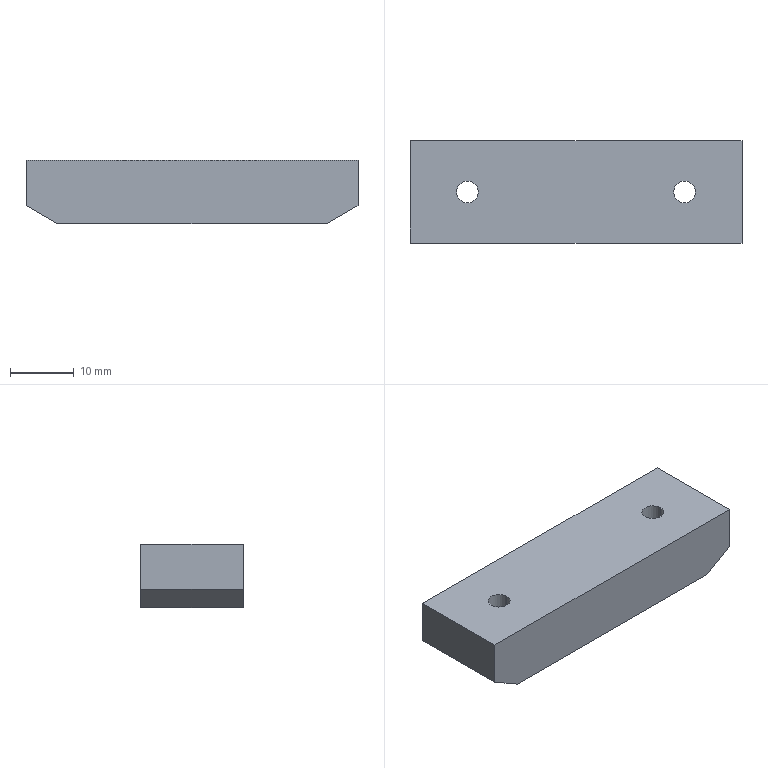Part | SolidWorks | features Chamfer 2, Extrusion 1, HoleWzd 1 | 1 solid | 18 faces | box 52 x 16 x 10 mm | volume 7777 mm3 | plane 10 | cylinder 8 | commonest cylinder face diameters 3.4 x4 6 x4
STEP:
#1=CARTESIAN_POINT('',(20.,0.,3.4));
#2=VERTEX_POINT('',#1);
#3=CARTESIAN_POINT('',(14.,0.,3.4));
#4=VERTEX_POINT('',#3);
#5=CARTESIAN_POINT('',(17.,0.,3.4));
#6=DIRECTION('',(0.,0.,-1.));
#7=DIRECTION('',(-1.,0.,0.));
#8=AXIS2_PLACEMENT_3D('',#5,#6,#7);
#9=CIRCLE('',#8,3.);
#10=EDGE_CURVE('',#2,#4,#9,.T.);
#11=ORIENTED_EDGE('',*,*,#10,.F.);
#12=CARTESIAN_POINT('',(20.,0.,0.));
#13=VERTEX_POINT('',#12);
#14=CARTESIAN_POINT('',(20.,0.,0.));
#15=DIRECTION('',(0.,0.,-1.));
#16=VECTOR('',#15,1000.);
#17=LINE('',#14,#16);
#18=EDGE_CURVE('',#2,#13,#17,.T.);
#19=ORIENTED_EDGE('',*,*,#18,.T.);
#20=CARTESIAN_POINT('',(14.,0.,0.));
#21=VERTEX_POINT('',#20);
#22=CARTESIAN_POINT('',(17.,0.,0.));
#23=DIRECTION('',(0.,0.,-1.));
#24=DIRECTION('',(-1.,0.,0.));
#25=AXIS2_PLACEMENT_3D('',#22,#23,#24);
#26=CIRCLE('',#25,3.);
#27=EDGE_CURVE('',#13,#21,#26,.T.);
#28=ORIENTED_EDGE('',*,*,#27,.T.);
#29=CARTESIAN_POINT('',(14.,0.,0.));
#30=DIRECTION('',(0.,0.,-1.));
#31=VECTOR('',#30,1000.);
#32=LINE('',#29,#31);
#33=EDGE_CURVE('',#4,#21,#32,.T.);
#34=ORIENTED_EDGE('',*,*,#33,.F.);
#35=EDGE_LOOP('',(#11,#19,#28,#34));
#36=FACE_OUTER_BOUND('',#35,.T.);
#37=CARTESIAN_POINT('',(17.,0.,0.));
#38=DIRECTION('',(0.,0.,-1.));
#39=DIRECTION('',(-1.,0.,0.));
#40=AXIS2_PLACEMENT_3D('',#37,#38,#39);
#41=CYLINDRICAL_SURFACE('',#40,3.);
#42=ADVANCED_FACE('',(#36),#41,.F.);
#43=CARTESIAN_POINT('',(15.3,0.,10.));
#44=VERTEX_POINT('',#43);
#45=CARTESIAN_POINT('',(18.7,0.,10.));
#46=VERTEX_POINT('',#45);
#47=CARTESIAN_POINT('',(17.,0.,10.));
#48=DIRECTION('',(0.,0.,1.));
#49=DIRECTION('',(1.,0.,0.));
#50=AXIS2_PLACEMENT_3D('',#47,#48,#49);
#51=CIRCLE('',#50,1.7);
#52=EDGE_CURVE('',#44,#46,#51,.T.);
#53=ORIENTED_EDGE('',*,*,#52,.T.);
#54=CARTESIAN_POINT('',(18.7,0.,3.4));
#55=VERTEX_POINT('',#54);
#56=CARTESIAN_POINT('',(18.7,0.,0.));
#57=DIRECTION('',(0.,0.,-1.));
#58=VECTOR('',#57,1000.);
#59=LINE('',#56,#58);
#60=EDGE_CURVE('',#46,#55,#59,.T.);
#61=ORIENTED_EDGE('',*,*,#60,.T.);
#62=CARTESIAN_POINT('',(15.3,0.,3.4));
#63=VERTEX_POINT('',#62);
#64=CARTESIAN_POINT('',(17.,0.,3.4));
#65=DIRECTION('',(0.,0.,-1.));
#66=DIRECTION('',(-1.,0.,0.));
#67=AXIS2_PLACEMENT_3D('',#64,#65,#66);
#68=CIRCLE('',#67,1.7);
#69=EDGE_CURVE('',#55,#63,#68,.T.);
#70=ORIENTED_EDGE('',*,*,#69,.T.);
#71=CARTESIAN_POINT('',(15.3,0.,0.));
#72=DIRECTION('',(0.,0.,-1.));
#73=VECTOR('',#72,1000.);
#74=LINE('',#71,#73);
#75=EDGE_CURVE('',#44,#63,#74,.T.);
#76=ORIENTED_EDGE('',*,*,#75,.F.);
#77=EDGE_LOOP('',(#53,#61,#70,#76));
#78=FACE_OUTER_BOUND('',#77,.T.);
#79=CARTESIAN_POINT('',(17.,0.,0.));
#80=DIRECTION('',(0.,0.,-1.));
#81=DIRECTION('',(-1.,0.,0.));
#82=AXIS2_PLACEMENT_3D('',#79,#80,#81);
#83=CYLINDRICAL_SURFACE('',#82,1.7);
#84=ADVANCED_FACE('',(#78),#83,.F.);
#85=CARTESIAN_POINT('',(-14.,0.,3.4));
#86=VERTEX_POINT('',#85);
#87=CARTESIAN_POINT('',(-20.,0.,3.4));
#88=VERTEX_POINT('',#87);
#89=CARTESIAN_POINT('',(-17.,0.,3.4));
#90=DIRECTION('',(0.,0.,-1.));
#91=DIRECTION('',(-1.,0.,0.));
#92=AXIS2_PLACEMENT_3D('',#89,#90,#91);
#93=CIRCLE('',#92,3.);
#94=EDGE_CURVE('',#86,#88,#93,.T.);
#95=ORIENTED_EDGE('',*,*,#94,.F.);
#96=CARTESIAN_POINT('',(-14.,0.,0.));
#97=VERTEX_POINT('',#96);
#98=CARTESIAN_POINT('',(-14.,0.,0.));
#99=DIRECTION('',(0.,0.,-1.));
#100=VECTOR('',#99,1000.);
#101=LINE('',#98,#100);
#102=EDGE_CURVE('',#86,#97,#101,.T.);
#103=ORIENTED_EDGE('',*,*,#102,.T.);
#104=CARTESIAN_POINT('',(-20.,0.,0.));
#105=VERTEX_POINT('',#104);
#106=CARTESIAN_POINT('',(-17.,0.,0.));
#107=DIRECTION('',(0.,0.,-1.));
#108=DIRECTION('',(-1.,0.,0.));
#109=AXIS2_PLACEMENT_3D('',#106,#107,#108);
#110=CIRCLE('',#109,3.);
#111=EDGE_CURVE('',#97,#105,#110,.T.);
#112=ORIENTED_EDGE('',*,*,#111,.T.);
#113=CARTESIAN_POINT('',(-20.,0.,0.));
#114=DIRECTION('',(0.,0.,-1.));
#115=VECTOR('',#114,1000.);
#116=LINE('',#113,#115);
#117=EDGE_CURVE('',#88,#105,#116,.T.);
#118=ORIENTED_EDGE('',*,*,#117,.F.);
#119=EDGE_LOOP('',(#95,#103,#112,#118));
#120=FACE_OUTER_BOUND('',#119,.T.);
#121=CARTESIAN_POINT('',(-17.,0.,0.));
#122=DIRECTION('',(0.,0.,-1.));
#123=DIRECTION('',(-1.,0.,0.));
#124=AXIS2_PLACEMENT_3D('',#121,#122,#123);
#125=CYLINDRICAL_SURFACE('',#124,3.);
#126=ADVANCED_FACE('',(#120),#125,.F.);
#127=CARTESIAN_POINT('',(-18.7,0.,10.));
#128=VERTEX_POINT('',#127);
#129=CARTESIAN_POINT('',(-15.3,0.,10.));
#130=VERTEX_POINT('',#129);
#131=CARTESIAN_POINT('',(-17.,0.,10.));
#132=DIRECTION('',(0.,0.,1.));
#133=DIRECTION('',(1.,0.,0.));
#134=AXIS2_PLACEMENT_3D('',#131,#132,#133);
#135=CIRCLE('',#134,1.7);
#136=EDGE_CURVE('',#128,#130,#135,.T.);
#137=ORIENTED_EDGE('',*,*,#136,.T.);
#138=CARTESIAN_POINT('',(-15.3,0.,3.4));
#139=VERTEX_POINT('',#138);
#140=CARTESIAN_POINT('',(-15.3,0.,0.));
#141=DIRECTION('',(0.,0.,-1.));
#142=VECTOR('',#141,1000.);
#143=LINE('',#140,#142);
#144=EDGE_CURVE('',#130,#139,#143,.T.);
#145=ORIENTED_EDGE('',*,*,#144,.T.);
#146=CARTESIAN_POINT('',(-18.7,0.,3.4));
#147=VERTEX_POINT('',#146);
#148=CARTESIAN_POINT('',(-17.,0.,3.4));
#149=DIRECTION('',(0.,0.,-1.));
#150=DIRECTION('',(-1.,0.,0.));
#151=AXIS2_PLACEMENT_3D('',#148,#149,#150);
#152=CIRCLE('',#151,1.7);
#153=EDGE_CURVE('',#139,#147,#152,.T.);
#154=ORIENTED_EDGE('',*,*,#153,.T.);
#155=CARTESIAN_POINT('',(-18.7,0.,0.));
#156=DIRECTION('',(0.,0.,-1.));
#157=VECTOR('',#156,1000.);
#158=LINE('',#155,#157);
#159=EDGE_CURVE('',#128,#147,#158,.T.);
#160=ORIENTED_EDGE('',*,*,#159,.F.);
#161=EDGE_LOOP('',(#137,#145,#154,#160));
#162=FACE_OUTER_BOUND('',#161,.T.);
#163=CARTESIAN_POINT('',(-17.,0.,0.));
#164=DIRECTION('',(0.,0.,-1.));
#165=DIRECTION('',(-1.,0.,0.));
#166=AXIS2_PLACEMENT_3D('',#163,#164,#165);
#167=CYLINDRICAL_SURFACE('',#166,1.7);
#168=ADVANCED_FACE('',(#162),#167,.F.);
#169=CARTESIAN_POINT('',(-26.,8.,10.));
#170=VERTEX_POINT('',#169);
#171=CARTESIAN_POINT('',(-26.,8.,2.887));
#172=VERTEX_POINT('',#171);
#173=CARTESIAN_POINT('',(-26.,8.,10.));
#174=DIRECTION('',(0.,0.,-1.));
#175=VECTOR('',#174,1000.);
#176=LINE('',#173,#175);
#177=EDGE_CURVE('',#170,#172,#176,.T.);
#178=ORIENTED_EDGE('',*,*,#177,.T.);
#179=CARTESIAN_POINT('',(-26.,-8.,2.887));
#180=VERTEX_POINT('',#179);
#181=CARTESIAN_POINT('',(-26.,-8.,2.887));
#182=DIRECTION('',(0.,-1.,0.));
#183=VECTOR('',#182,1000.);
#184=LINE('',#181,#183);
#185=EDGE_CURVE('',#172,#180,#184,.T.);
#186=ORIENTED_EDGE('',*,*,#185,.T.);
#187=CARTESIAN_POINT('',(-26.,-8.,10.));
#188=VERTEX_POINT('',#187);
#189=CARTESIAN_POINT('',(-26.,-8.,10.));
#190=DIRECTION('',(0.,0.,-1.));
#191=VECTOR('',#190,1000.);
#192=LINE('',#189,#191);
#193=EDGE_CURVE('',#188,#180,#192,.T.);
#194=ORIENTED_EDGE('',*,*,#193,.F.);
#195=CARTESIAN_POINT('',(-26.,-8.,10.));
#196=DIRECTION('',(0.,-1.,0.));
#197=VECTOR('',#196,1000.);
#198=LINE('',#195,#197);
#199=EDGE_CURVE('',#170,#188,#198,.T.);
#200=ORIENTED_EDGE('',*,*,#199,.F.);
#201=EDGE_LOOP('',(#178,#186,#194,#200));
#202=FACE_OUTER_BOUND('',#201,.T.);
#203=CARTESIAN_POINT('',(-26.,-8.,10.));
#204=DIRECTION('',(1.,0.,0.));
#205=DIRECTION('',(0.,0.,-1.));
#206=AXIS2_PLACEMENT_3D('',#203,#204,#205);
#207=PLANE('',#206);
#208=ADVANCED_FACE('',(#202),#207,.F.);
#209=ORIENTED_EDGE('',*,*,#193,.T.);
#210=CARTESIAN_POINT('',(-21.,-8.,0.));
#211=VERTEX_POINT('',#210);
#212=CARTESIAN_POINT('',(-26.,-8.,2.887));
#213=DIRECTION('',(0.866,0.,-0.5));
#214=VECTOR('',#213,1000.);
#215=LINE('',#212,#214);
#216=EDGE_CURVE('',#180,#211,#215,.T.);
#217=ORIENTED_EDGE('',*,*,#216,.T.);
#218=CARTESIAN_POINT('',(21.,-8.,0.));
#219=VERTEX_POINT('',#218);
#220=CARTESIAN_POINT('',(26.,-8.,0.));
#221=DIRECTION('',(1.,0.,0.));
#222=VECTOR('',#221,1000.);
#223=LINE('',#220,#222);
#224=EDGE_CURVE('',#211,#219,#223,.T.);
#225=ORIENTED_EDGE('',*,*,#224,.T.);
#226=CARTESIAN_POINT('',(26.,-8.,2.887));
#227=VERTEX_POINT('',#226);
#228=CARTESIAN_POINT('',(26.,-8.,2.887));
#229=DIRECTION('',(0.866,0.,0.5));
#230=VECTOR('',#229,1000.);
#231=LINE('',#228,#230);
#232=EDGE_CURVE('',#219,#227,#231,.T.);
#233=ORIENTED_EDGE('',*,*,#232,.T.);
#234=CARTESIAN_POINT('',(26.,-8.,10.));
#235=VERTEX_POINT('',#234);
#236=CARTESIAN_POINT('',(26.,-8.,10.));
#237=DIRECTION('',(0.,0.,-1.));
#238=VECTOR('',#237,1000.);
#239=LINE('',#236,#238);
#240=EDGE_CURVE('',#235,#227,#239,.T.);
#241=ORIENTED_EDGE('',*,*,#240,.F.);
#242=CARTESIAN_POINT('',(26.,-8.,10.));
#243=DIRECTION('',(1.,0.,0.));
#244=VECTOR('',#243,1000.);
#245=LINE('',#242,#244);
#246=EDGE_CURVE('',#188,#235,#245,.T.);
#247=ORIENTED_EDGE('',*,*,#246,.F.);
#248=EDGE_LOOP('',(#209,#217,#225,#233,#241,#247));
#249=FACE_OUTER_BOUND('',#248,.T.);
#250=CARTESIAN_POINT('',(26.,-8.,10.));
#251=DIRECTION('',(0.,1.,0.));
#252=DIRECTION('',(-1.,0.,0.));
#253=AXIS2_PLACEMENT_3D('',#250,#251,#252);
#254=PLANE('',#253);
#255=ADVANCED_FACE('',(#249),#254,.F.);
#256=ORIENTED_EDGE('',*,*,#240,.T.);
#257=CARTESIAN_POINT('',(26.,8.,2.887));
#258=VERTEX_POINT('',#257);
#259=CARTESIAN_POINT('',(26.,-8.,2.887));
#260=DIRECTION('',(0.,1.,0.));
#261=VECTOR('',#260,1000.);
#262=LINE('',#259,#261);
#263=EDGE_CURVE('',#227,#258,#262,.T.);
#264=ORIENTED_EDGE('',*,*,#263,.T.);
#265=CARTESIAN_POINT('',(26.,8.,10.));
#266=VERTEX_POINT('',#265);
#267=CARTESIAN_POINT('',(26.,8.,10.));
#268=DIRECTION('',(0.,0.,-1.));
#269=VECTOR('',#268,1000.);
#270=LINE('',#267,#269);
#271=EDGE_CURVE('',#266,#258,#270,.T.);
#272=ORIENTED_EDGE('',*,*,#271,.F.);
#273=CARTESIAN_POINT('',(26.,-8.,10.));
#274=DIRECTION('',(0.,1.,0.));
#275=VECTOR('',#274,1000.);
#276=LINE('',#273,#275);
#277=EDGE_CURVE('',#235,#266,#276,.T.);
#278=ORIENTED_EDGE('',*,*,#277,.F.);
#279=EDGE_LOOP('',(#256,#264,#272,#278));
#280=FACE_OUTER_BOUND('',#279,.T.);
#281=CARTESIAN_POINT('',(26.,-8.,10.));
#282=DIRECTION('',(-1.,0.,0.));
#283=DIRECTION('',(0.,0.,1.));
#284=AXIS2_PLACEMENT_3D('',#281,#282,#283);
#285=PLANE('',#284);
#286=ADVANCED_FACE('',(#280),#285,.F.);
#287=CARTESIAN_POINT('',(21.,8.,0.));
#288=VERTEX_POINT('',#287);
#289=CARTESIAN_POINT('',(-21.,8.,0.));
#290=VERTEX_POINT('',#289);
#291=CARTESIAN_POINT('',(26.,8.,0.));
#292=DIRECTION('',(-1.,0.,0.));
#293=VECTOR('',#292,1000.);
#294=LINE('',#291,#293);
#295=EDGE_CURVE('',#288,#290,#294,.T.);
#296=ORIENTED_EDGE('',*,*,#295,.T.);
#297=CARTESIAN_POINT('',(-26.,8.,2.887));
#298=DIRECTION('',(-0.866,0.,0.5));
#299=VECTOR('',#298,1000.);
#300=LINE('',#297,#299);
#301=EDGE_CURVE('',#290,#172,#300,.T.);
#302=ORIENTED_EDGE('',*,*,#301,.T.);
#303=ORIENTED_EDGE('',*,*,#177,.F.);
#304=CARTESIAN_POINT('',(26.,8.,10.));
#305=DIRECTION('',(-1.,0.,0.));
#306=VECTOR('',#305,1000.);
#307=LINE('',#304,#306);
#308=EDGE_CURVE('',#266,#170,#307,.T.);
#309=ORIENTED_EDGE('',*,*,#308,.F.);
#310=ORIENTED_EDGE('',*,*,#271,.T.);
#311=CARTESIAN_POINT('',(26.,8.,2.887));
#312=DIRECTION('',(-0.866,0.,-0.5));
#313=VECTOR('',#312,1000.);
#314=LINE('',#311,#313);
#315=EDGE_CURVE('',#258,#288,#314,.T.);
#316=ORIENTED_EDGE('',*,*,#315,.T.);
#317=EDGE_LOOP('',(#296,#302,#303,#309,#310,#316));
#318=FACE_OUTER_BOUND('',#317,.T.);
#319=CARTESIAN_POINT('',(26.,8.,10.));
#320=DIRECTION('',(0.,-1.,0.));
#321=DIRECTION('',(1.,0.,0.));
#322=AXIS2_PLACEMENT_3D('',#319,#320,#321);
#323=PLANE('',#322);
#324=ADVANCED_FACE('',(#318),#323,.F.);
#325=ORIENTED_EDGE('',*,*,#52,.F.);
#326=CARTESIAN_POINT('',(17.,0.,10.));
#327=DIRECTION('',(0.,0.,1.));
#328=DIRECTION('',(1.,0.,0.));
#329=AXIS2_PLACEMENT_3D('',#326,#327,#328);
#330=CIRCLE('',#329,1.7);
#331=EDGE_CURVE('',#46,#44,#330,.T.);
#332=ORIENTED_EDGE('',*,*,#331,.F.);
#333=EDGE_LOOP('',(#325,#332));
#334=FACE_BOUND('',#333,.T.);
#335=ORIENTED_EDGE('',*,*,#136,.F.);
#336=CARTESIAN_POINT('',(-17.,0.,10.));
#337=DIRECTION('',(0.,0.,1.));
#338=DIRECTION('',(1.,0.,0.));
#339=AXIS2_PLACEMENT_3D('',#336,#337,#338);
#340=CIRCLE('',#339,1.7);
#341=EDGE_CURVE('',#130,#128,#340,.T.);
#342=ORIENTED_EDGE('',*,*,#341,.F.);
#343=EDGE_LOOP('',(#335,#342));
#344=FACE_BOUND('',#343,.T.);
#345=ORIENTED_EDGE('',*,*,#199,.T.);
#346=ORIENTED_EDGE('',*,*,#246,.T.);
#347=ORIENTED_EDGE('',*,*,#277,.T.);
#348=ORIENTED_EDGE('',*,*,#308,.T.);
#349=EDGE_LOOP('',(#345,#346,#347,#348));
#350=FACE_OUTER_BOUND('',#349,.T.);
#351=CARTESIAN_POINT('',(0.,0.,10.));
#352=DIRECTION('',(0.,0.,1.));
#353=DIRECTION('',(1.,0.,0.));
#354=AXIS2_PLACEMENT_3D('',#351,#352,#353);
#355=PLANE('',#354);
#356=ADVANCED_FACE('',(#334,#344,#350),#355,.T.);
#357=CARTESIAN_POINT('',(17.,0.,0.));
#358=DIRECTION('',(0.,0.,-1.));
#359=DIRECTION('',(-1.,0.,0.));
#360=AXIS2_PLACEMENT_3D('',#357,#358,#359);
#361=CIRCLE('',#360,3.);
#362=EDGE_CURVE('',#21,#13,#361,.T.);
#363=ORIENTED_EDGE('',*,*,#362,.F.);
#364=ORIENTED_EDGE('',*,*,#27,.F.);
#365=EDGE_LOOP('',(#363,#364));
#366=FACE_BOUND('',#365,.T.);
#367=CARTESIAN_POINT('',(-17.,0.,0.));
#368=DIRECTION('',(0.,0.,-1.));
#369=DIRECTION('',(-1.,0.,0.));
#370=AXIS2_PLACEMENT_3D('',#367,#368,#369);
#371=CIRCLE('',#370,3.);
#372=EDGE_CURVE('',#105,#97,#371,.T.);
#373=ORIENTED_EDGE('',*,*,#372,.F.);
#374=ORIENTED_EDGE('',*,*,#111,.F.);
#375=EDGE_LOOP('',(#373,#374));
#376=FACE_BOUND('',#375,.T.);
#377=ORIENTED_EDGE('',*,*,#224,.F.);
#378=CARTESIAN_POINT('',(-21.,0.,0.));
#379=DIRECTION('',(0.,1.,0.));
#380=VECTOR('',#379,1000.);
#381=LINE('',#378,#380);
#382=EDGE_CURVE('',#211,#290,#381,.T.);
#383=ORIENTED_EDGE('',*,*,#382,.T.);
#384=ORIENTED_EDGE('',*,*,#295,.F.);
#385=CARTESIAN_POINT('',(21.,0.,0.));
#386=DIRECTION('',(0.,-1.,0.));
#387=VECTOR('',#386,1000.);
#388=LINE('',#385,#387);
#389=EDGE_CURVE('',#288,#219,#388,.T.);
#390=ORIENTED_EDGE('',*,*,#389,.T.);
#391=EDGE_LOOP('',(#377,#383,#384,#390));
#392=FACE_OUTER_BOUND('',#391,.T.);
#393=CARTESIAN_POINT('',(0.,0.,0.));
#394=DIRECTION('',(0.,0.,1.));
#395=DIRECTION('',(1.,0.,0.));
#396=AXIS2_PLACEMENT_3D('',#393,#394,#395);
#397=PLANE('',#396);
#398=ADVANCED_FACE('',(#366,#376,#392),#397,.F.);
#399=ORIENTED_EDGE('',*,*,#144,.F.);
#400=ORIENTED_EDGE('',*,*,#341,.T.);
#401=ORIENTED_EDGE('',*,*,#159,.T.);
#402=CARTESIAN_POINT('',(-17.,0.,3.4));
#403=DIRECTION('',(0.,0.,-1.));
#404=DIRECTION('',(-1.,0.,0.));
#405=AXIS2_PLACEMENT_3D('',#402,#403,#404);
#406=CIRCLE('',#405,1.7);
#407=EDGE_CURVE('',#147,#139,#406,.T.);
#408=ORIENTED_EDGE('',*,*,#407,.T.);
#409=EDGE_LOOP('',(#399,#400,#401,#408));
#410=FACE_OUTER_BOUND('',#409,.T.);
#411=CARTESIAN_POINT('',(-17.,0.,0.));
#412=DIRECTION('',(0.,0.,-1.));
#413=DIRECTION('',(-1.,0.,0.));
#414=AXIS2_PLACEMENT_3D('',#411,#412,#413);
#415=CYLINDRICAL_SURFACE('',#414,1.7);
#416=ADVANCED_FACE('',(#410),#415,.F.);
#417=ORIENTED_EDGE('',*,*,#407,.F.);
#418=ORIENTED_EDGE('',*,*,#153,.F.);
#419=EDGE_LOOP('',(#417,#418));
#420=FACE_BOUND('',#419,.T.);
#421=CARTESIAN_POINT('',(-17.,0.,3.4));
#422=DIRECTION('',(0.,0.,-1.));
#423=DIRECTION('',(-1.,0.,0.));
#424=AXIS2_PLACEMENT_3D('',#421,#422,#423);
#425=CIRCLE('',#424,3.);
#426=EDGE_CURVE('',#88,#86,#425,.T.);
#427=ORIENTED_EDGE('',*,*,#426,.T.);
#428=ORIENTED_EDGE('',*,*,#94,.T.);
#429=EDGE_LOOP('',(#427,#428));
#430=FACE_OUTER_BOUND('',#429,.T.);
#431=CARTESIAN_POINT('',(-15.3,0.,3.4));
#432=DIRECTION('',(0.,0.,1.));
#433=DIRECTION('',(1.,0.,0.));
#434=AXIS2_PLACEMENT_3D('',#431,#432,#433);
#435=PLANE('',#434);
#436=ADVANCED_FACE('',(#420,#430),#435,.F.);
#437=ORIENTED_EDGE('',*,*,#102,.F.);
#438=ORIENTED_EDGE('',*,*,#426,.F.);
#439=ORIENTED_EDGE('',*,*,#117,.T.);
#440=ORIENTED_EDGE('',*,*,#372,.T.);
#441=EDGE_LOOP('',(#437,#438,#439,#440));
#442=FACE_OUTER_BOUND('',#441,.T.);
#443=CARTESIAN_POINT('',(-17.,0.,0.));
#444=DIRECTION('',(0.,0.,-1.));
#445=DIRECTION('',(-1.,0.,0.));
#446=AXIS2_PLACEMENT_3D('',#443,#444,#445);
#447=CYLINDRICAL_SURFACE('',#446,3.);
#448=ADVANCED_FACE('',(#442),#447,.F.);
#449=ORIENTED_EDGE('',*,*,#60,.F.);
#450=ORIENTED_EDGE('',*,*,#331,.T.);
#451=ORIENTED_EDGE('',*,*,#75,.T.);
#452=CARTESIAN_POINT('',(17.,0.,3.4));
#453=DIRECTION('',(0.,0.,-1.));
#454=DIRECTION('',(-1.,0.,0.));
#455=AXIS2_PLACEMENT_3D('',#452,#453,#454);
#456=CIRCLE('',#455,1.7);
#457=EDGE_CURVE('',#63,#55,#456,.T.);
#458=ORIENTED_EDGE('',*,*,#457,.T.);
#459=EDGE_LOOP('',(#449,#450,#451,#458));
#460=FACE_OUTER_BOUND('',#459,.T.);
#461=CARTESIAN_POINT('',(17.,0.,0.));
#462=DIRECTION('',(0.,0.,-1.));
#463=DIRECTION('',(-1.,0.,0.));
#464=AXIS2_PLACEMENT_3D('',#461,#462,#463);
#465=CYLINDRICAL_SURFACE('',#464,1.7);
#466=ADVANCED_FACE('',(#460),#465,.F.);
#467=ORIENTED_EDGE('',*,*,#457,.F.);
#468=ORIENTED_EDGE('',*,*,#69,.F.);
#469=EDGE_LOOP('',(#467,#468));
#470=FACE_BOUND('',#469,.T.);
#471=CARTESIAN_POINT('',(17.,0.,3.4));
#472=DIRECTION('',(0.,0.,-1.));
#473=DIRECTION('',(-1.,0.,0.));
#474=AXIS2_PLACEMENT_3D('',#471,#472,#473);
#475=CIRCLE('',#474,3.);
#476=EDGE_CURVE('',#4,#2,#475,.T.);
#477=ORIENTED_EDGE('',*,*,#476,.T.);
#478=ORIENTED_EDGE('',*,*,#10,.T.);
#479=EDGE_LOOP('',(#477,#478));
#480=FACE_OUTER_BOUND('',#479,.T.);
#481=CARTESIAN_POINT('',(18.7,0.,3.4));
#482=DIRECTION('',(0.,0.,1.));
#483=DIRECTION('',(1.,0.,0.));
#484=AXIS2_PLACEMENT_3D('',#481,#482,#483);
#485=PLANE('',#484);
#486=ADVANCED_FACE('',(#470,#480),#485,.F.);
#487=ORIENTED_EDGE('',*,*,#18,.F.);
#488=ORIENTED_EDGE('',*,*,#476,.F.);
#489=ORIENTED_EDGE('',*,*,#33,.T.);
#490=ORIENTED_EDGE('',*,*,#362,.T.);
#491=EDGE_LOOP('',(#487,#488,#489,#490));
#492=FACE_OUTER_BOUND('',#491,.T.);
#493=CARTESIAN_POINT('',(17.,0.,0.));
#494=DIRECTION('',(0.,0.,-1.));
#495=DIRECTION('',(-1.,0.,0.));
#496=AXIS2_PLACEMENT_3D('',#493,#494,#495);
#497=CYLINDRICAL_SURFACE('',#496,3.);
#498=ADVANCED_FACE('',(#492),#497,.F.);
#499=ORIENTED_EDGE('',*,*,#232,.F.);
#500=ORIENTED_EDGE('',*,*,#389,.F.);
#501=ORIENTED_EDGE('',*,*,#315,.F.);
#502=ORIENTED_EDGE('',*,*,#263,.F.);
#503=EDGE_LOOP('',(#499,#500,#501,#502));
#504=FACE_OUTER_BOUND('',#503,.T.);
#505=CARTESIAN_POINT('',(26.,-8.,2.887));
#506=DIRECTION('',(-0.5,0.,0.866));
#507=DIRECTION('',(0.,1.,0.));
#508=AXIS2_PLACEMENT_3D('',#505,#506,#507);
#509=PLANE('',#508);
#510=ADVANCED_FACE('',(#504),#509,.F.);
#511=ORIENTED_EDGE('',*,*,#301,.F.);
#512=ORIENTED_EDGE('',*,*,#382,.F.);
#513=ORIENTED_EDGE('',*,*,#216,.F.);
#514=ORIENTED_EDGE('',*,*,#185,.F.);
#515=EDGE_LOOP('',(#511,#512,#513,#514));
#516=FACE_OUTER_BOUND('',#515,.T.);
#517=CARTESIAN_POINT('',(-26.,-8.,2.887));
#518=DIRECTION('',(0.5,0.,0.866));
#519=DIRECTION('',(0.,-1.,0.));
#520=AXIS2_PLACEMENT_3D('',#517,#518,#519);
#521=PLANE('',#520);
#522=ADVANCED_FACE('',(#516),#521,.F.);
#523=CLOSED_SHELL('',(#42,#84,#126,#168,#208,#255,#286,#324,#356,#398,#416,#436,#448,#466,#486,#498,#510,#522));
#524=MANIFOLD_SOLID_BREP('',#523);
#525=CARTESIAN_POINT('',(0.,0.,0.));
#526=DIRECTION('',(0.,0.,1.));
#527=DIRECTION('',(1.,0.,0.));
#528=AXIS2_PLACEMENT_3D('',#525,#526,#527);
#529=(LENGTH_UNIT()NAMED_UNIT(*)SI_UNIT(.MILLI.,.METRE.));
#530=UNCERTAINTY_MEASURE_WITH_UNIT(LENGTH_MEASURE(0.00001),#529,'','');
#531=(NAMED_UNIT(*)PLANE_ANGLE_UNIT()SI_UNIT($,.RADIAN.));
#532=(NAMED_UNIT(*)SI_UNIT($,.STERADIAN.)SOLID_ANGLE_UNIT());
#533=(GEOMETRIC_REPRESENTATION_CONTEXT(3)GLOBAL_UNCERTAINTY_ASSIGNED_CONTEXT((#530))GLOBAL_UNIT_ASSIGNED_CONTEXT((#529,#531,#532))REPRESENTATION_CONTEXT('',''));
#534=ADVANCED_BREP_SHAPE_REPRESENTATION('',(#524,#528),#533);